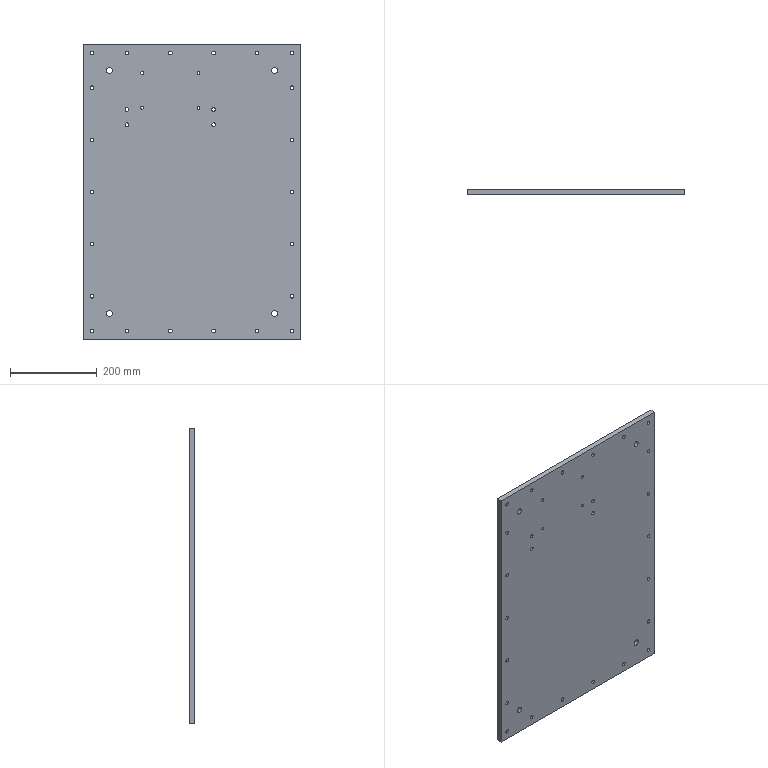Part | STEP file | PN_0014 (base plate) | 1 solid | 74 faces | box 500 x 12 x 680 mm | volume 4053163 mm3 | cylinder 68 | plane 6 | commonest cylinder face diameters 8.5 x52 6.8 x8 14 x8